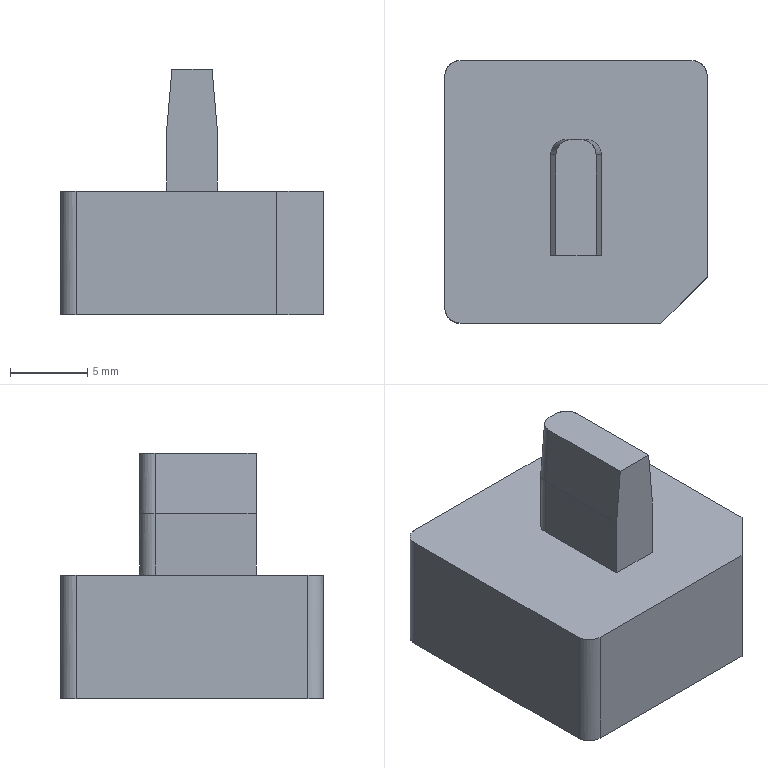CAM job | PowerMill | 3-axis milling, other | part box 17 x 17 x 15.883 mm
Tools:
number,name,type,diameter,tip_radius,length,cutting_length,overhang,flutes,holder,toolpaths_using
1,D10C_1_1,end_mill,10.0,0.0,60.0,,16.32,1,D42L35,6
3,D10_1_1,end_mill,10.0,0.0,60.0,,16.04,1,D42L35,6
14,D4_1_1,end_mill,4.0,0.0,30.0,,8.04,1,D42L35,2
13,Text_D4_1_1,taper_spherical,4.0,0.3,60.0,,8.16,1,D42L35,2
14,D4_2_1,end_mill,4.0,0.0,30.0,,7.92,1,D42L35,2
Operations:
program,toolpath,strategy,tool,tool_number,tool_diameter,tip_radius,flutes,spindle_rpm,feed_cut,surface_speed_m_min_computed,feed_per_tooth_computed,tolerance,thickness,stepover,stepdown,cut_length,cut_time_min,total_time_min,workplane
29-C01-5-F,精公开粗01-扫面平行-D10C,raster_area_clear,D10C_1_1,1,10.0,0.0,1.0,8000.0,10000.0,251.33,1.25,0.03,0.28,6.0,1.0,135.36,0.013,0.0178,
29-C01-5-F,精公开粗01-外形偏置-D10C,offset_area_clear,D10C_1_1,1,10.0,0.0,1.0,8000.0,10000.0,251.33,1.25,0.03,0.28,6.0,1.0,2968.495,0.297,0.3477,
29-C01-5-F,精公开粗01-基准台等高-D10C,constantz,D10C_1_1,1,10.0,0.0,1.0,8000.0,10000.0,251.33,1.25,0.03,0.07,5.0,0.4,2129.104,0.213,0.2213,
29-C01-5-F,精公基准台01-平坦面偏置-D10,offset_area_clear,D10_1_1,3,10.0,0.0,1.0,8500.0,600.0,267.04,0.0706,0.005,0.38,5.0,1.0,26.956,0.045,0.0606,
29-C01-5-F,精公基准台01-基准面偏置-D10,offset_area_clear,D10_1_1,3,10.0,0.0,1.0,8500.0,600.0,267.04,0.0706,0.005,0.38,5.0,1.0,64.791,0.108,0.1256,
29-C01-5-F,精公基准台01-基准台侧光-D10,profile_area_clear,D10_1_1,3,10.0,0.0,1.0,8500.0,600.0,267.04,0.0706,0.005,0.0,0.08,1.0,193.234,0.322,0.3849,
29-C01-5-F,精公精光01-等高-D4,constantz,D4_1_1,14,4.0,0.0,1.0,18000.0,2000.0,226.19,0.1111,0.005,-0.075,5.0,0.04,6406.563,3.203,3.209,
29-C01-5-F,精公精光01-平坦面偏置-D4,offset_area_clear,D4_1_1,14,4.0,0.0,1.0,18000.0,600.0,226.19,0.0333,0.005,0.375,2.0,1.0,24.367,0.041,0.0504,
29-C01-5-F,精公刻字01-刻字-Text_D4,pattern,Text_D4_1_1,13,4.0,0.3,1.0,15000.0,1000.0,188.5,0.0667,0.005,0.0,5.0,1.0,28.683,0.029,0.0447,
29-C01-5-R,粗公开粗01-扫面平行-D10C,raster_area_clear,D10C_1_1,1,10.0,0.0,1.0,8000.0,10000.0,251.33,1.25,0.03,0.15,6.0,1.0,133.8,0.013,0.0185,
29-C01-5-R,粗公开粗01-外形偏置-D10C,offset_area_clear,D10C_1_1,1,10.0,0.0,1.0,8000.0,10000.0,251.33,1.25,0.03,0.15,6.0,1.0,2931.777,0.293,0.3443,
29-C01-5-R,粗公开粗01-基准台等高-D10C,constantz,D10C_1_1,1,10.0,0.0,1.0,8000.0,10000.0,251.33,1.25,0.03,0.07,5.0,0.4,2129.104,0.213,0.2213,
29-C01-5-R,粗公基准台01-平坦面偏置-D10,offset_area_clear,D10_1_1,3,10.0,0.0,1.0,8500.0,600.0,267.04,0.0706,0.01,0.25,5.0,1.0,25.901,0.043,0.0588,
29-C01-5-R,粗公基准台01-基准面偏置-D10,offset_area_clear,D10_1_1,3,10.0,0.0,1.0,8500.0,600.0,267.04,0.0706,0.01,0.25,5.0,1.0,64.628,0.108,0.1255,
29-C01-5-R,粗公基准台01-基准台侧光-D10,profile_area_clear,D10_1_1,3,10.0,0.0,1.0,8500.0,600.0,267.04,0.0706,0.01,0.0,0.08,1.0,193.218,0.322,0.3849,
29-C01-5-R,粗公精光01-等高-D4,constantz,D4_2_1,14,4.0,0.0,1.0,18000.0,2000.0,226.19,0.1111,0.01,-0.205,5.0,0.048,5104.021,2.552,2.558,
29-C01-5-R,粗公精光01-平坦面偏置-D4,offset_area_clear,D4_2_1,14,4.0,0.0,1.0,18000.0,600.0,226.19,0.0333,0.01,0.245,2.0,1.0,23.463,0.039,0.0489,
29-C01-5-R,粗公刻字01-刻字-Text_D4,pattern,Text_D4_1_1,13,4.0,0.3,1.0,15000.0,1000.0,188.5,0.0667,0.01,0.0,5.0,1.0,28.835,0.029,0.0441,